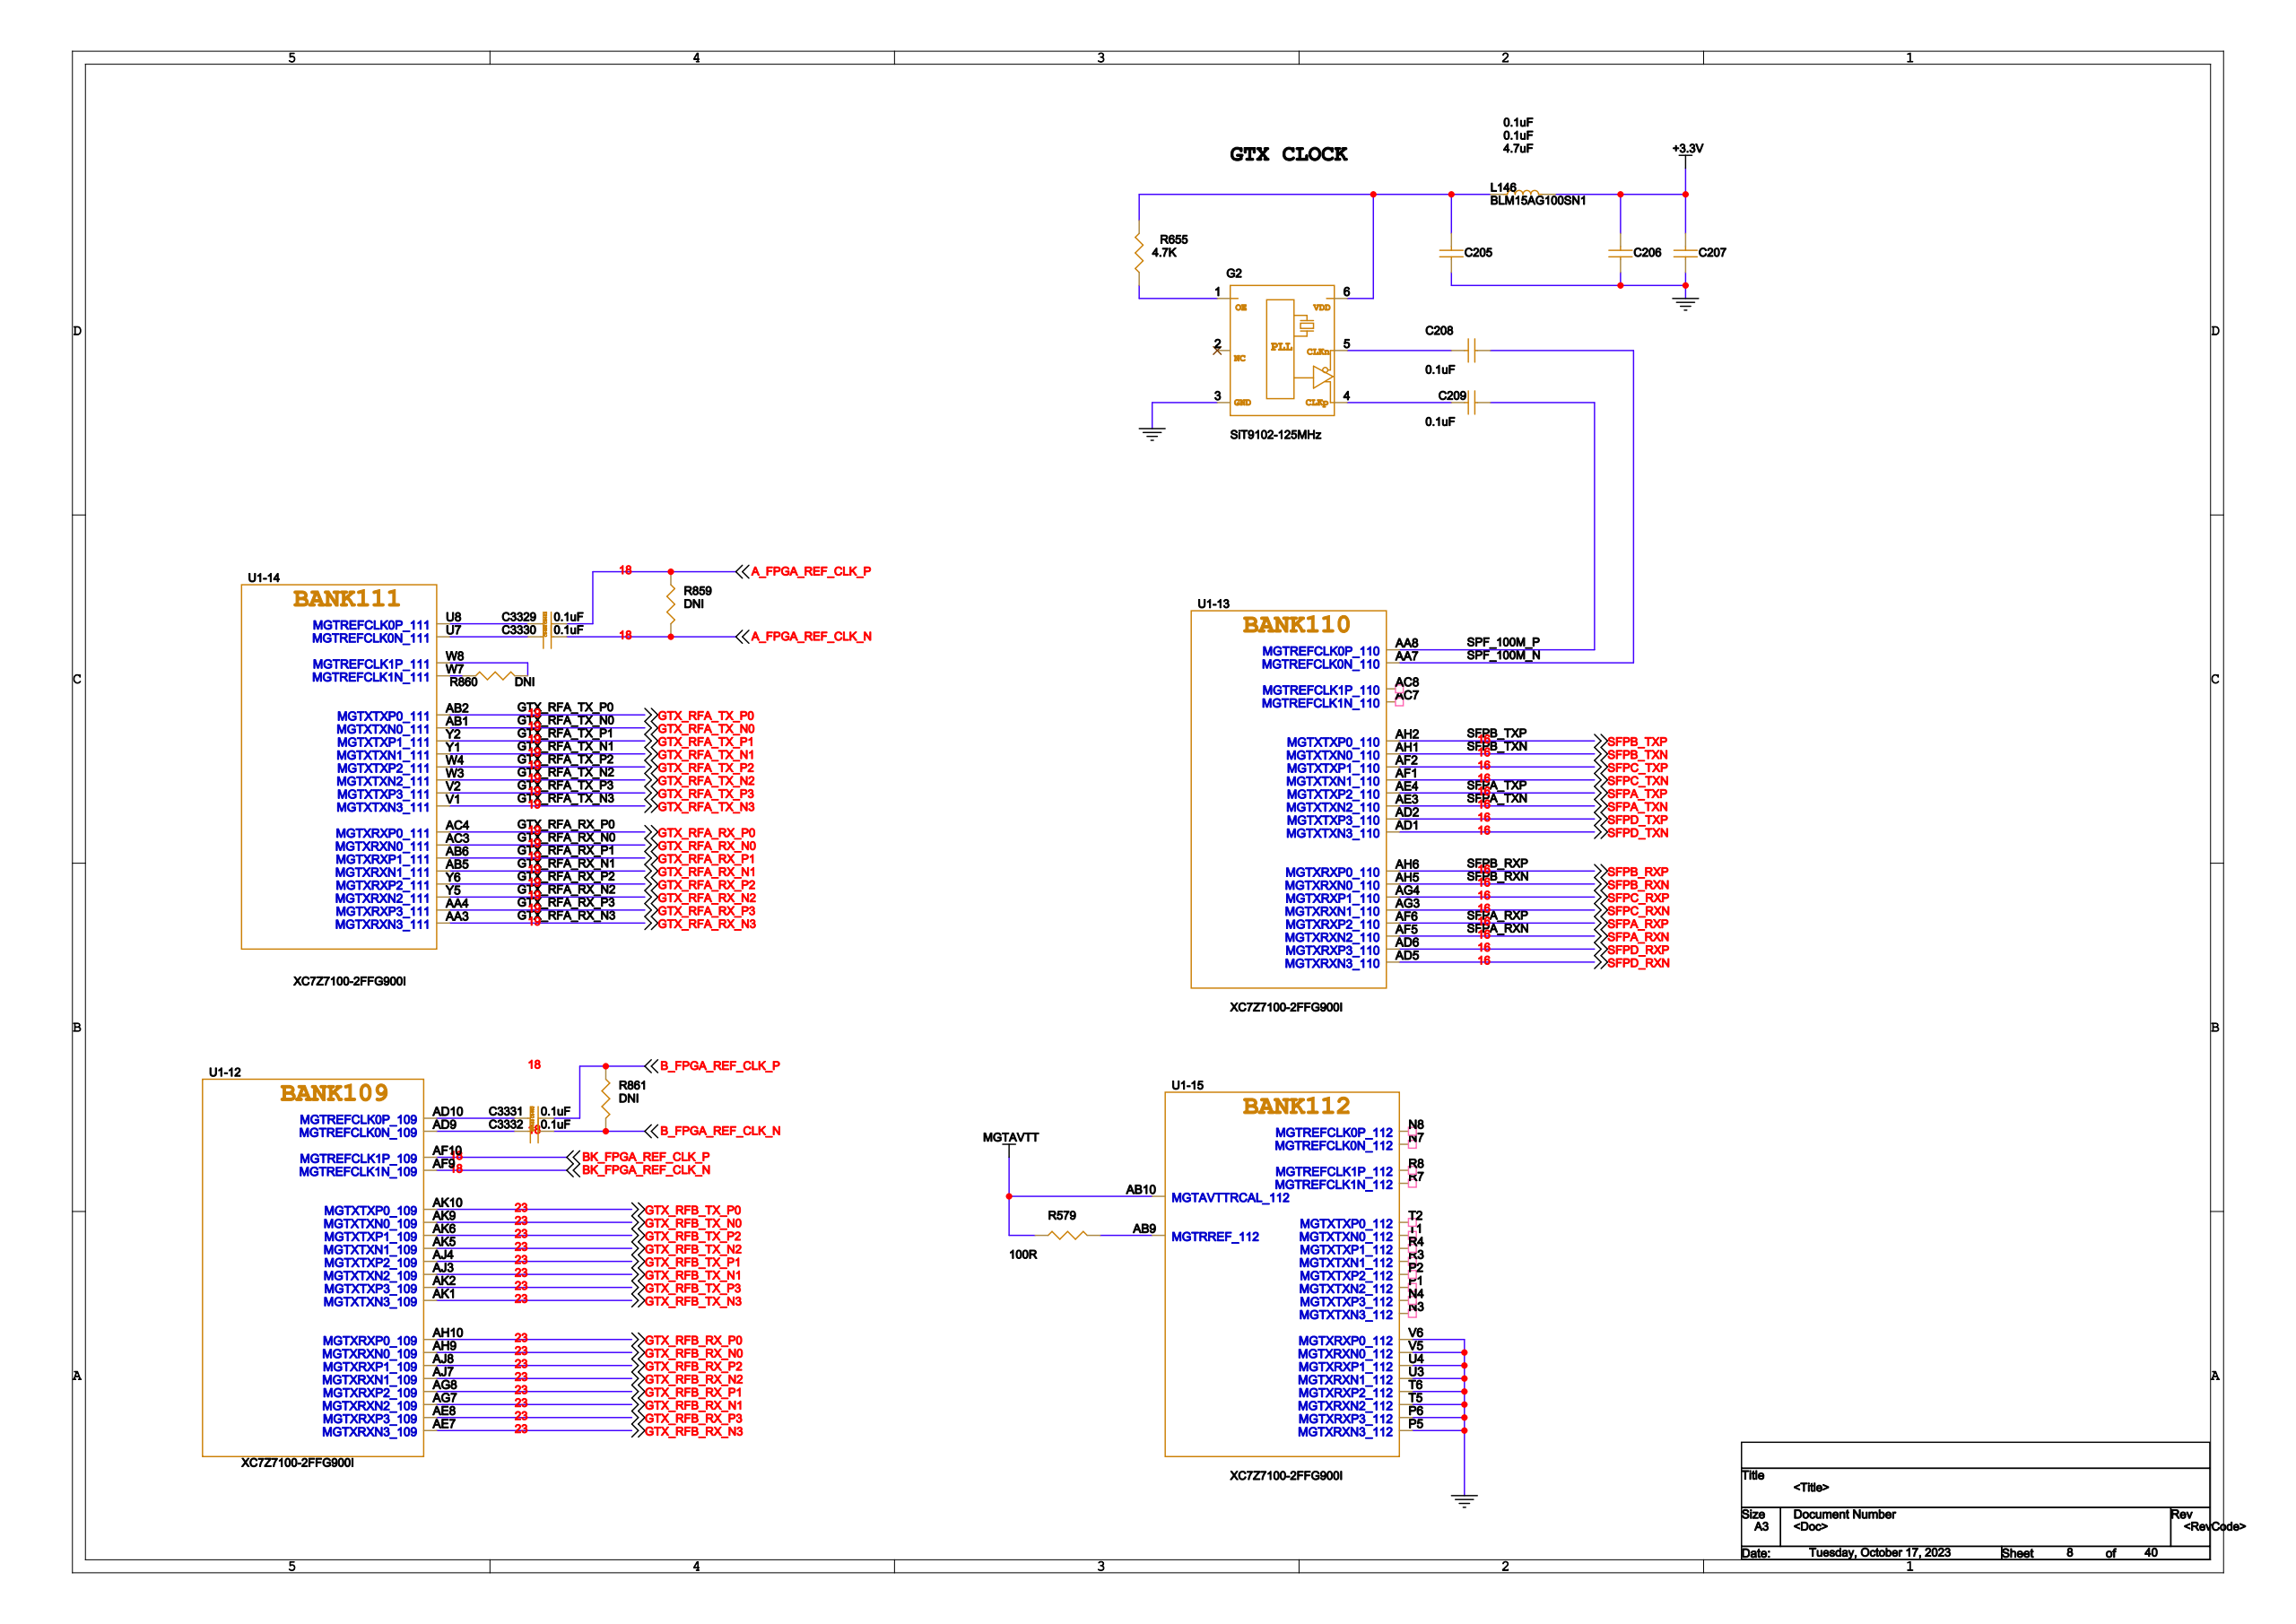Circuit board | Cadence Allegro | 1793 parts | 1223 nets | one sheet of the schematic
Parts on this sheet (reference | value | footprint):
AD1 | AD9371 | BGA196
AD2 | AD9371 | BGA196
C205 | 0.1uF | C0402
C206 | 0.1uF | C0402
C207 | 4.7uF | C0402
C208 | 0.1uF | C0402
C209 | 0.1uF | C0402
C3329 | 0.1uF | C0402
C3330 | 0.1uF | C0402
C3331 | 0.1uF | C0402
C3332 | 0.1uF | C0402
G2 | SiT9102-125MHz | OSC6-3225
L146 | BLM15AG100SN1 | L0402
R579 | 100R | R0402
R655 | 4.7K | R0402
R859 | DNI | R0402
R860 | DNI | R0402
R861 | DNI | R0402
U3 | MYMGM1R824ELA5RA | MYMGM1R
U4 | MT41J256M16 | FBGA-96
U7 | MT41J256M16 | FBGA-96
U8 | MT41J256M16 | FBGA-96
Nets of these parts (net: part-pin ...):
GND: C205-1 C206-1 C207-1 G2-3 AD1-G2 AD1-N7 AD1-P1 AD1-P2 AD2-G2 AD2-N7 AD2-P1 AD2-P2 U3-G2 U4-P1 U4-T1 U7-P1 U7-T1 U8-P1 U8-T1
+3.3V: C206-2 C207-2 L146-2
MGTAVTT: R579-2
N16992270: C208-2 G2-5
N16992291: C209-2 G2-4
N16992231: G2-1 R655-2
N16992173: C205-2 G2-6 L146-1 R655-1
N47590: R579-1
SPF_100M_N: C208-1
SPF_100M_P: C209-1
N16913210: C3329-1
A_FPGA_REF_CLK_P: C3329-2 R859-2
N16913207: C3330-1
A_FPGA_REF_CLK_N: C3330-2 R859-1
N18809356: C3331-1
B_FPGA_REF_CLK_P: C3331-2 R861-2
N18809380: C3332-1
B_FPGA_REF_CLK_N: C3332-2 R861-1
N16913273: R860-1
N16913270: R860-2